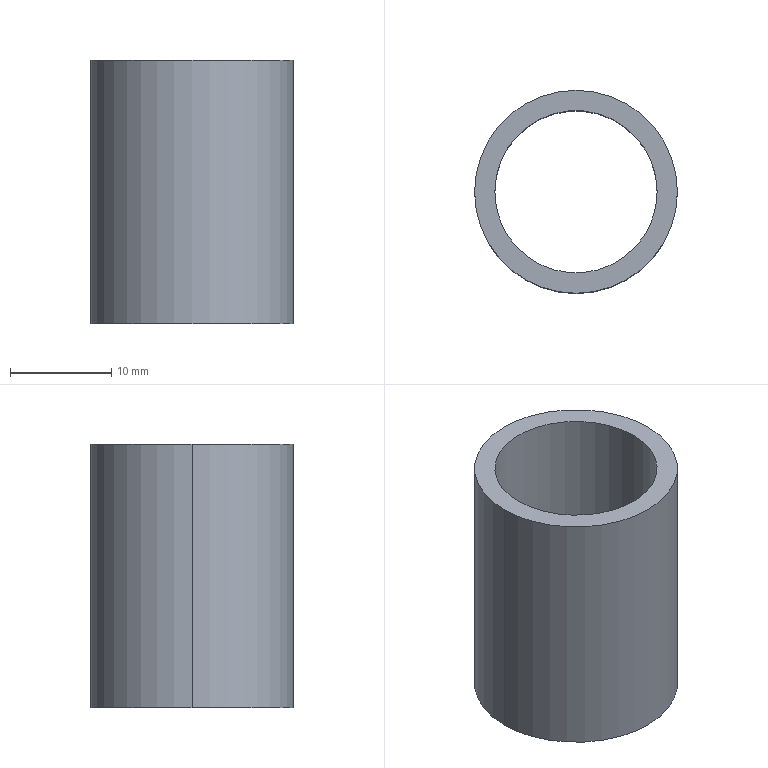Part | SolidWorks | features Extrusion 1 | 1 solid | 6 faces | box 20 x 20 x 26 mm | volume 2941 mm3 | cylinder 4 | plane 2 | commonest cylinder face diameters 16 x2 20 x2
STEP:
#1=CARTESIAN_POINT('',(-8.,0.,13.));
#2=VERTEX_POINT('',#1);
#3=CARTESIAN_POINT('',(8.,0.,13.));
#4=VERTEX_POINT('',#3);
#5=CARTESIAN_POINT('',(0.,0.,13.));
#6=DIRECTION('',(0.,0.,1.));
#7=DIRECTION('',(1.,0.,0.));
#8=AXIS2_PLACEMENT_3D('',#5,#6,#7);
#9=CIRCLE('',#8,8.);
#10=EDGE_CURVE('',#2,#4,#9,.T.);
#11=ORIENTED_EDGE('',*,*,#10,.T.);
#12=CARTESIAN_POINT('',(8.,0.,-13.));
#13=VERTEX_POINT('',#12);
#14=CARTESIAN_POINT('',(8.,0.,13.));
#15=DIRECTION('',(0.,0.,-1.));
#16=VECTOR('',#15,1000.);
#17=LINE('',#14,#16);
#18=EDGE_CURVE('',#4,#13,#17,.T.);
#19=ORIENTED_EDGE('',*,*,#18,.T.);
#20=CARTESIAN_POINT('',(-8.,0.,-13.));
#21=VERTEX_POINT('',#20);
#22=CARTESIAN_POINT('',(0.,0.,-13.));
#23=DIRECTION('',(0.,0.,1.));
#24=DIRECTION('',(1.,0.,0.));
#25=AXIS2_PLACEMENT_3D('',#22,#23,#24);
#26=CIRCLE('',#25,8.);
#27=EDGE_CURVE('',#21,#13,#26,.T.);
#28=ORIENTED_EDGE('',*,*,#27,.F.);
#29=CARTESIAN_POINT('',(-8.,0.,13.));
#30=DIRECTION('',(0.,0.,-1.));
#31=VECTOR('',#30,1000.);
#32=LINE('',#29,#31);
#33=EDGE_CURVE('',#2,#21,#32,.T.);
#34=ORIENTED_EDGE('',*,*,#33,.F.);
#35=EDGE_LOOP('',(#11,#19,#28,#34));
#36=FACE_OUTER_BOUND('',#35,.T.);
#37=CARTESIAN_POINT('',(0.,0.,13.));
#38=DIRECTION('',(0.,0.,-1.));
#39=DIRECTION('',(-1.,0.,0.));
#40=AXIS2_PLACEMENT_3D('',#37,#38,#39);
#41=CYLINDRICAL_SURFACE('',#40,8.);
#42=ADVANCED_FACE('',(#36),#41,.F.);
#43=CARTESIAN_POINT('',(10.,0.,13.));
#44=VERTEX_POINT('',#43);
#45=CARTESIAN_POINT('',(-10.,0.,13.));
#46=VERTEX_POINT('',#45);
#47=CARTESIAN_POINT('',(0.,0.,13.));
#48=DIRECTION('',(0.,0.,1.));
#49=DIRECTION('',(1.,0.,0.));
#50=AXIS2_PLACEMENT_3D('',#47,#48,#49);
#51=CIRCLE('',#50,10.);
#52=EDGE_CURVE('',#44,#46,#51,.T.);
#53=ORIENTED_EDGE('',*,*,#52,.F.);
#54=CARTESIAN_POINT('',(10.,0.,-13.));
#55=VERTEX_POINT('',#54);
#56=CARTESIAN_POINT('',(10.,0.,13.));
#57=DIRECTION('',(0.,0.,-1.));
#58=VECTOR('',#57,1000.);
#59=LINE('',#56,#58);
#60=EDGE_CURVE('',#44,#55,#59,.T.);
#61=ORIENTED_EDGE('',*,*,#60,.T.);
#62=CARTESIAN_POINT('',(-10.,0.,-13.));
#63=VERTEX_POINT('',#62);
#64=CARTESIAN_POINT('',(0.,0.,-13.));
#65=DIRECTION('',(0.,0.,1.));
#66=DIRECTION('',(1.,0.,0.));
#67=AXIS2_PLACEMENT_3D('',#64,#65,#66);
#68=CIRCLE('',#67,10.);
#69=EDGE_CURVE('',#55,#63,#68,.T.);
#70=ORIENTED_EDGE('',*,*,#69,.T.);
#71=CARTESIAN_POINT('',(-10.,0.,13.));
#72=DIRECTION('',(0.,0.,-1.));
#73=VECTOR('',#72,1000.);
#74=LINE('',#71,#73);
#75=EDGE_CURVE('',#46,#63,#74,.T.);
#76=ORIENTED_EDGE('',*,*,#75,.F.);
#77=EDGE_LOOP('',(#53,#61,#70,#76));
#78=FACE_OUTER_BOUND('',#77,.T.);
#79=CARTESIAN_POINT('',(0.,0.,13.));
#80=DIRECTION('',(0.,0.,-1.));
#81=DIRECTION('',(-1.,0.,0.));
#82=AXIS2_PLACEMENT_3D('',#79,#80,#81);
#83=CYLINDRICAL_SURFACE('',#82,10.);
#84=ADVANCED_FACE('',(#78),#83,.T.);
#85=CARTESIAN_POINT('',(0.,0.,13.));
#86=DIRECTION('',(0.,0.,1.));
#87=DIRECTION('',(1.,0.,0.));
#88=AXIS2_PLACEMENT_3D('',#85,#86,#87);
#89=CIRCLE('',#88,10.);
#90=EDGE_CURVE('',#46,#44,#89,.T.);
#91=ORIENTED_EDGE('',*,*,#90,.T.);
#92=ORIENTED_EDGE('',*,*,#52,.T.);
#93=EDGE_LOOP('',(#91,#92));
#94=FACE_OUTER_BOUND('',#93,.T.);
#95=ORIENTED_EDGE('',*,*,#10,.F.);
#96=CARTESIAN_POINT('',(0.,0.,13.));
#97=DIRECTION('',(0.,0.,1.));
#98=DIRECTION('',(1.,0.,0.));
#99=AXIS2_PLACEMENT_3D('',#96,#97,#98);
#100=CIRCLE('',#99,8.);
#101=EDGE_CURVE('',#4,#2,#100,.T.);
#102=ORIENTED_EDGE('',*,*,#101,.F.);
#103=EDGE_LOOP('',(#95,#102));
#104=FACE_BOUND('',#103,.T.);
#105=CARTESIAN_POINT('',(0.,0.,13.));
#106=DIRECTION('',(0.,0.,1.));
#107=DIRECTION('',(1.,0.,0.));
#108=AXIS2_PLACEMENT_3D('',#105,#106,#107);
#109=PLANE('',#108);
#110=ADVANCED_FACE('',(#94,#104),#109,.T.);
#111=CARTESIAN_POINT('',(0.,0.,-13.));
#112=DIRECTION('',(0.,0.,1.));
#113=DIRECTION('',(1.,0.,0.));
#114=AXIS2_PLACEMENT_3D('',#111,#112,#113);
#115=CIRCLE('',#114,10.);
#116=EDGE_CURVE('',#63,#55,#115,.T.);
#117=ORIENTED_EDGE('',*,*,#116,.F.);
#118=ORIENTED_EDGE('',*,*,#69,.F.);
#119=EDGE_LOOP('',(#117,#118));
#120=FACE_OUTER_BOUND('',#119,.T.);
#121=ORIENTED_EDGE('',*,*,#27,.T.);
#122=CARTESIAN_POINT('',(0.,0.,-13.));
#123=DIRECTION('',(0.,0.,1.));
#124=DIRECTION('',(1.,0.,0.));
#125=AXIS2_PLACEMENT_3D('',#122,#123,#124);
#126=CIRCLE('',#125,8.);
#127=EDGE_CURVE('',#13,#21,#126,.T.);
#128=ORIENTED_EDGE('',*,*,#127,.T.);
#129=EDGE_LOOP('',(#121,#128));
#130=FACE_BOUND('',#129,.T.);
#131=CARTESIAN_POINT('',(0.,0.,-13.));
#132=DIRECTION('',(0.,0.,1.));
#133=DIRECTION('',(1.,0.,0.));
#134=AXIS2_PLACEMENT_3D('',#131,#132,#133);
#135=PLANE('',#134);
#136=ADVANCED_FACE('',(#120,#130),#135,.F.);
#137=ORIENTED_EDGE('',*,*,#60,.F.);
#138=ORIENTED_EDGE('',*,*,#90,.F.);
#139=ORIENTED_EDGE('',*,*,#75,.T.);
#140=ORIENTED_EDGE('',*,*,#116,.T.);
#141=EDGE_LOOP('',(#137,#138,#139,#140));
#142=FACE_OUTER_BOUND('',#141,.T.);
#143=CARTESIAN_POINT('',(0.,0.,13.));
#144=DIRECTION('',(0.,0.,-1.));
#145=DIRECTION('',(-1.,0.,0.));
#146=AXIS2_PLACEMENT_3D('',#143,#144,#145);
#147=CYLINDRICAL_SURFACE('',#146,10.);
#148=ADVANCED_FACE('',(#142),#147,.T.);
#149=ORIENTED_EDGE('',*,*,#18,.F.);
#150=ORIENTED_EDGE('',*,*,#101,.T.);
#151=ORIENTED_EDGE('',*,*,#33,.T.);
#152=ORIENTED_EDGE('',*,*,#127,.F.);
#153=EDGE_LOOP('',(#149,#150,#151,#152));
#154=FACE_OUTER_BOUND('',#153,.T.);
#155=CARTESIAN_POINT('',(0.,0.,13.));
#156=DIRECTION('',(0.,0.,-1.));
#157=DIRECTION('',(-1.,0.,0.));
#158=AXIS2_PLACEMENT_3D('',#155,#156,#157);
#159=CYLINDRICAL_SURFACE('',#158,8.);
#160=ADVANCED_FACE('',(#154),#159,.F.);
#161=CLOSED_SHELL('',(#42,#84,#110,#136,#148,#160));
#162=MANIFOLD_SOLID_BREP('',#161);
#163=CARTESIAN_POINT('',(0.,0.,0.));
#164=DIRECTION('',(0.,0.,1.));
#165=DIRECTION('',(1.,0.,0.));
#166=AXIS2_PLACEMENT_3D('',#163,#164,#165);
#167=(LENGTH_UNIT()NAMED_UNIT(*)SI_UNIT(.MILLI.,.METRE.));
#168=UNCERTAINTY_MEASURE_WITH_UNIT(LENGTH_MEASURE(0.00001),#167,'','');
#169=(NAMED_UNIT(*)PLANE_ANGLE_UNIT()SI_UNIT($,.RADIAN.));
#170=(NAMED_UNIT(*)SI_UNIT($,.STERADIAN.)SOLID_ANGLE_UNIT());
#171=(GEOMETRIC_REPRESENTATION_CONTEXT(3)GLOBAL_UNCERTAINTY_ASSIGNED_CONTEXT((#168))GLOBAL_UNIT_ASSIGNED_CONTEXT((#167,#169,#170))REPRESENTATION_CONTEXT('',''));
#172=ADVANCED_BREP_SHAPE_REPRESENTATION('',(#162,#166),#171);